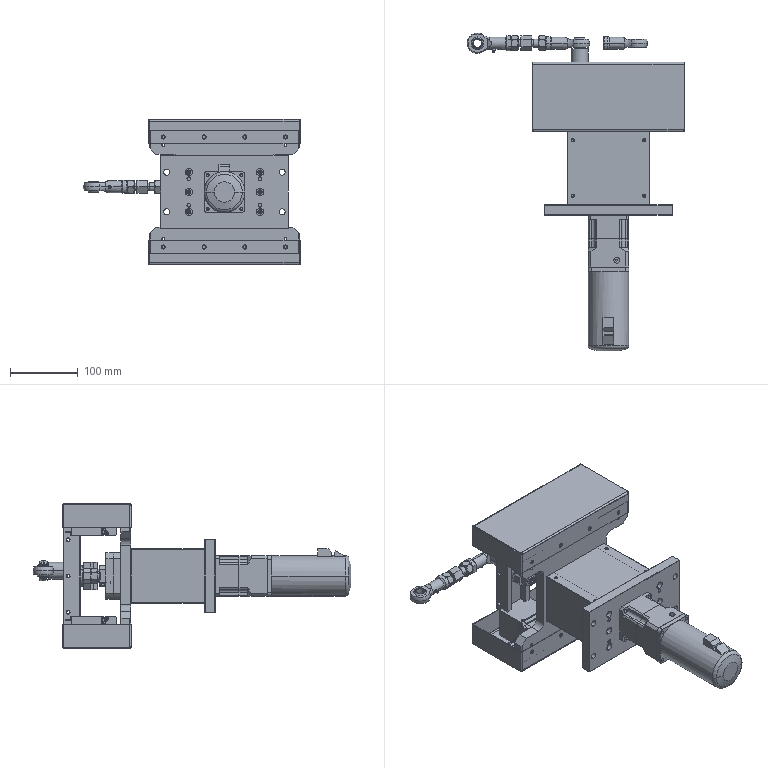Part | NX | 71 solids | 3832 faces | volume 2646697 mm3 | plane 1771 | cylinder 1374 | cone 506 | torus 129 | spline 28 | sphere 24 | commonest cylinder face diameters 5 x142 3 x100 6.5 x96 3.5 x80 3.3 x64 4 x54